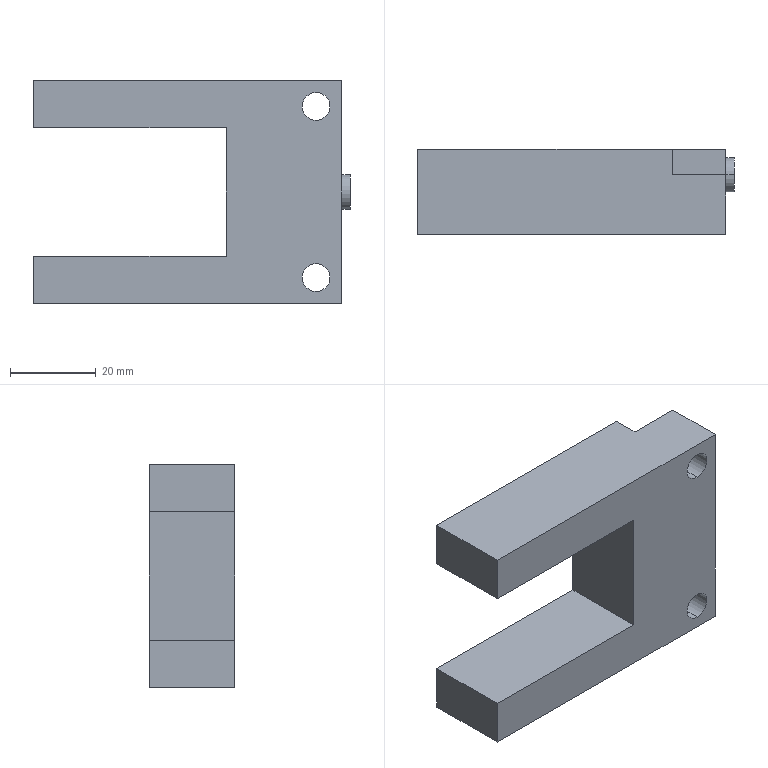Part | 1 solid | 23 faces | box 74 x 20 x 52 mm | volume 45176 mm3 | plane 17 | cylinder 6 | commonest cylinder face diameters 6.5 x4 8 x2
STEP:
#1=CARTESIAN_POINT('',(38.,14.,-4.));
#2=VERTEX_POINT('',#1);
#3=CARTESIAN_POINT('',(38.,14.,4.));
#4=VERTEX_POINT('',#3);
#5=CARTESIAN_POINT('',(38.,14.,0.));
#6=DIRECTION('',(1.,0.,0.));
#7=DIRECTION('',(0.,0.,-1.));
#8=AXIS2_PLACEMENT_3D('',#5,#6,#7);
#9=CIRCLE('',#8,4.);
#10=EDGE_CURVE('',#2,#4,#9,.T.);
#11=ORIENTED_EDGE('',*,*,#10,.F.);
#12=CARTESIAN_POINT('',(36.,14.,-4.));
#13=VERTEX_POINT('',#12);
#14=CARTESIAN_POINT('',(38.,14.,-4.));
#15=DIRECTION('',(-1.,0.,0.));
#16=VECTOR('',#15,1000.);
#17=LINE('',#14,#16);
#18=EDGE_CURVE('',#2,#13,#17,.T.);
#19=ORIENTED_EDGE('',*,*,#18,.T.);
#20=CARTESIAN_POINT('',(36.,14.,4.));
#21=VERTEX_POINT('',#20);
#22=CARTESIAN_POINT('',(36.,14.,0.));
#23=DIRECTION('',(1.,0.,0.));
#24=DIRECTION('',(0.,0.,1.));
#25=AXIS2_PLACEMENT_3D('',#22,#23,#24);
#26=CIRCLE('',#25,4.);
#27=EDGE_CURVE('',#13,#21,#26,.T.);
#28=ORIENTED_EDGE('',*,*,#27,.T.);
#29=CARTESIAN_POINT('',(38.,14.,4.));
#30=DIRECTION('',(-1.,0.,0.));
#31=VECTOR('',#30,1000.);
#32=LINE('',#29,#31);
#33=EDGE_CURVE('',#4,#21,#32,.T.);
#34=ORIENTED_EDGE('',*,*,#33,.F.);
#35=EDGE_LOOP('',(#11,#19,#28,#34));
#36=FACE_OUTER_BOUND('',#35,.T.);
#37=CARTESIAN_POINT('',(38.,14.,0.));
#38=DIRECTION('',(-1.,0.,0.));
#39=DIRECTION('',(0.,0.,1.));
#40=AXIS2_PLACEMENT_3D('',#37,#38,#39);
#41=CYLINDRICAL_SURFACE('',#40,4.);
#42=ADVANCED_FACE('',(#36),#41,.T.);
#43=CARTESIAN_POINT('',(30.,0.,-16.75));
#44=VERTEX_POINT('',#43);
#45=CARTESIAN_POINT('',(30.,0.,-23.25));
#46=VERTEX_POINT('',#45);
#47=CARTESIAN_POINT('',(30.,0.,-20.));
#48=DIRECTION('',(0.,-1.,0.));
#49=DIRECTION('',(0.,0.,-1.));
#50=AXIS2_PLACEMENT_3D('',#47,#48,#49);
#51=CIRCLE('',#50,3.25);
#52=EDGE_CURVE('',#44,#46,#51,.T.);
#53=ORIENTED_EDGE('',*,*,#52,.T.);
#54=CARTESIAN_POINT('',(30.,14.,-23.25));
#55=VERTEX_POINT('',#54);
#56=CARTESIAN_POINT('',(30.,14.,-23.25));
#57=DIRECTION('',(0.,1.,0.));
#58=VECTOR('',#57,1000.);
#59=LINE('',#56,#58);
#60=EDGE_CURVE('',#46,#55,#59,.T.);
#61=ORIENTED_EDGE('',*,*,#60,.T.);
#62=CARTESIAN_POINT('',(30.,14.,-16.75));
#63=VERTEX_POINT('',#62);
#64=CARTESIAN_POINT('',(30.,14.,-20.));
#65=DIRECTION('',(0.,1.,0.));
#66=DIRECTION('',(0.,0.,1.));
#67=AXIS2_PLACEMENT_3D('',#64,#65,#66);
#68=CIRCLE('',#67,3.25);
#69=EDGE_CURVE('',#55,#63,#68,.T.);
#70=ORIENTED_EDGE('',*,*,#69,.T.);
#71=CARTESIAN_POINT('',(30.,14.,-16.75));
#72=DIRECTION('',(0.,1.,0.));
#73=VECTOR('',#72,1000.);
#74=LINE('',#71,#73);
#75=EDGE_CURVE('',#44,#63,#74,.T.);
#76=ORIENTED_EDGE('',*,*,#75,.F.);
#77=EDGE_LOOP('',(#53,#61,#70,#76));
#78=FACE_OUTER_BOUND('',#77,.T.);
#79=CARTESIAN_POINT('',(30.,14.,-20.));
#80=DIRECTION('',(0.,1.,0.));
#81=DIRECTION('',(0.,0.,1.));
#82=AXIS2_PLACEMENT_3D('',#79,#80,#81);
#83=CYLINDRICAL_SURFACE('',#82,3.25);
#84=ADVANCED_FACE('',(#78),#83,.F.);
#85=CARTESIAN_POINT('',(30.,0.,23.25));
#86=VERTEX_POINT('',#85);
#87=CARTESIAN_POINT('',(30.,0.,16.75));
#88=VERTEX_POINT('',#87);
#89=CARTESIAN_POINT('',(30.,0.,20.));
#90=DIRECTION('',(0.,-1.,0.));
#91=DIRECTION('',(0.,0.,-1.));
#92=AXIS2_PLACEMENT_3D('',#89,#90,#91);
#93=CIRCLE('',#92,3.25);
#94=EDGE_CURVE('',#86,#88,#93,.T.);
#95=ORIENTED_EDGE('',*,*,#94,.T.);
#96=CARTESIAN_POINT('',(30.,14.,16.75));
#97=VERTEX_POINT('',#96);
#98=CARTESIAN_POINT('',(30.,14.,16.75));
#99=DIRECTION('',(0.,1.,0.));
#100=VECTOR('',#99,1000.);
#101=LINE('',#98,#100);
#102=EDGE_CURVE('',#88,#97,#101,.T.);
#103=ORIENTED_EDGE('',*,*,#102,.T.);
#104=CARTESIAN_POINT('',(30.,14.,23.25));
#105=VERTEX_POINT('',#104);
#106=CARTESIAN_POINT('',(30.,14.,20.));
#107=DIRECTION('',(0.,1.,0.));
#108=DIRECTION('',(0.,0.,1.));
#109=AXIS2_PLACEMENT_3D('',#106,#107,#108);
#110=CIRCLE('',#109,3.25);
#111=EDGE_CURVE('',#97,#105,#110,.T.);
#112=ORIENTED_EDGE('',*,*,#111,.T.);
#113=CARTESIAN_POINT('',(30.,14.,23.25));
#114=DIRECTION('',(0.,1.,0.));
#115=VECTOR('',#114,1000.);
#116=LINE('',#113,#115);
#117=EDGE_CURVE('',#86,#105,#116,.T.);
#118=ORIENTED_EDGE('',*,*,#117,.F.);
#119=EDGE_LOOP('',(#95,#103,#112,#118));
#120=FACE_OUTER_BOUND('',#119,.T.);
#121=CARTESIAN_POINT('',(30.,14.,20.));
#122=DIRECTION('',(0.,1.,0.));
#123=DIRECTION('',(0.,0.,1.));
#124=AXIS2_PLACEMENT_3D('',#121,#122,#123);
#125=CYLINDRICAL_SURFACE('',#124,3.25);
#126=ADVANCED_FACE('',(#120),#125,.F.);
#127=CARTESIAN_POINT('',(-36.,0.,-26.));
#128=VERTEX_POINT('',#127);
#129=CARTESIAN_POINT('',(-36.,0.,-15.));
#130=VERTEX_POINT('',#129);
#131=CARTESIAN_POINT('',(-36.,0.,26.));
#132=DIRECTION('',(0.,0.,1.));
#133=VECTOR('',#132,1000.);
#134=LINE('',#131,#133);
#135=EDGE_CURVE('',#128,#130,#134,.T.);
#136=ORIENTED_EDGE('',*,*,#135,.T.);
#137=CARTESIAN_POINT('',(-36.,20.,-15.));
#138=VERTEX_POINT('',#137);
#139=CARTESIAN_POINT('',(-36.,0.,-15.));
#140=DIRECTION('',(0.,1.,0.));
#141=VECTOR('',#140,1000.);
#142=LINE('',#139,#141);
#143=EDGE_CURVE('',#130,#138,#142,.T.);
#144=ORIENTED_EDGE('',*,*,#143,.T.);
#145=CARTESIAN_POINT('',(-36.,20.,-26.));
#146=VERTEX_POINT('',#145);
#147=CARTESIAN_POINT('',(-36.,20.,26.));
#148=DIRECTION('',(0.,0.,1.));
#149=VECTOR('',#148,1000.);
#150=LINE('',#147,#149);
#151=EDGE_CURVE('',#146,#138,#150,.T.);
#152=ORIENTED_EDGE('',*,*,#151,.F.);
#153=CARTESIAN_POINT('',(-36.,20.,-26.));
#154=DIRECTION('',(0.,-1.,0.));
#155=VECTOR('',#154,1000.);
#156=LINE('',#153,#155);
#157=EDGE_CURVE('',#146,#128,#156,.T.);
#158=ORIENTED_EDGE('',*,*,#157,.T.);
#159=EDGE_LOOP('',(#136,#144,#152,#158));
#160=FACE_OUTER_BOUND('',#159,.T.);
#161=CARTESIAN_POINT('',(-36.,20.,26.));
#162=DIRECTION('',(1.,0.,0.));
#163=DIRECTION('',(0.,0.,-1.));
#164=AXIS2_PLACEMENT_3D('',#161,#162,#163);
#165=PLANE('',#164);
#166=ADVANCED_FACE('',(#160),#165,.F.);
#167=CARTESIAN_POINT('',(36.,14.,0.));
#168=DIRECTION('',(1.,0.,0.));
#169=DIRECTION('',(0.,0.,1.));
#170=AXIS2_PLACEMENT_3D('',#167,#168,#169);
#171=CIRCLE('',#170,4.);
#172=EDGE_CURVE('',#21,#13,#171,.T.);
#173=ORIENTED_EDGE('',*,*,#172,.F.);
#174=ORIENTED_EDGE('',*,*,#27,.F.);
#175=EDGE_LOOP('',(#173,#174));
#176=FACE_BOUND('',#175,.T.);
#177=CARTESIAN_POINT('',(36.,14.,-13.5));
#178=VERTEX_POINT('',#177);
#179=CARTESIAN_POINT('',(36.,14.,-26.));
#180=VERTEX_POINT('',#179);
#181=CARTESIAN_POINT('',(36.,14.,-26.));
#182=DIRECTION('',(0.,0.,-1.));
#183=VECTOR('',#182,1000.);
#184=LINE('',#181,#183);
#185=EDGE_CURVE('',#178,#180,#184,.T.);
#186=ORIENTED_EDGE('',*,*,#185,.F.);
#187=CARTESIAN_POINT('',(36.,20.,-13.5));
#188=VERTEX_POINT('',#187);
#189=CARTESIAN_POINT('',(36.,14.,-13.5));
#190=DIRECTION('',(0.,1.,0.));
#191=VECTOR('',#190,1000.);
#192=LINE('',#189,#191);
#193=EDGE_CURVE('',#178,#188,#192,.T.);
#194=ORIENTED_EDGE('',*,*,#193,.T.);
#195=CARTESIAN_POINT('',(36.,20.,13.5));
#196=VERTEX_POINT('',#195);
#197=CARTESIAN_POINT('',(36.,20.,26.));
#198=DIRECTION('',(0.,0.,-1.));
#199=VECTOR('',#198,1000.);
#200=LINE('',#197,#199);
#201=EDGE_CURVE('',#196,#188,#200,.T.);
#202=ORIENTED_EDGE('',*,*,#201,.F.);
#203=CARTESIAN_POINT('',(36.,14.,13.5));
#204=VERTEX_POINT('',#203);
#205=CARTESIAN_POINT('',(36.,14.,13.5));
#206=DIRECTION('',(0.,1.,0.));
#207=VECTOR('',#206,1000.);
#208=LINE('',#205,#207);
#209=EDGE_CURVE('',#204,#196,#208,.T.);
#210=ORIENTED_EDGE('',*,*,#209,.F.);
#211=CARTESIAN_POINT('',(36.,14.,26.));
#212=VERTEX_POINT('',#211);
#213=CARTESIAN_POINT('',(36.,14.,26.));
#214=DIRECTION('',(0.,0.,-1.));
#215=VECTOR('',#214,1000.);
#216=LINE('',#213,#215);
#217=EDGE_CURVE('',#212,#204,#216,.T.);
#218=ORIENTED_EDGE('',*,*,#217,.F.);
#219=CARTESIAN_POINT('',(36.,0.,26.));
#220=VERTEX_POINT('',#219);
#221=CARTESIAN_POINT('',(36.,20.,26.));
#222=DIRECTION('',(0.,-1.,0.));
#223=VECTOR('',#222,1000.);
#224=LINE('',#221,#223);
#225=EDGE_CURVE('',#212,#220,#224,.T.);
#226=ORIENTED_EDGE('',*,*,#225,.T.);
#227=CARTESIAN_POINT('',(36.,0.,-26.));
#228=VERTEX_POINT('',#227);
#229=CARTESIAN_POINT('',(36.,0.,26.));
#230=DIRECTION('',(0.,0.,-1.));
#231=VECTOR('',#230,1000.);
#232=LINE('',#229,#231);
#233=EDGE_CURVE('',#220,#228,#232,.T.);
#234=ORIENTED_EDGE('',*,*,#233,.T.);
#235=CARTESIAN_POINT('',(36.,20.,-26.));
#236=DIRECTION('',(0.,-1.,0.));
#237=VECTOR('',#236,1000.);
#238=LINE('',#235,#237);
#239=EDGE_CURVE('',#180,#228,#238,.T.);
#240=ORIENTED_EDGE('',*,*,#239,.F.);
#241=EDGE_LOOP('',(#186,#194,#202,#210,#218,#226,#234,#240));
#242=FACE_OUTER_BOUND('',#241,.T.);
#243=CARTESIAN_POINT('',(36.,20.,26.));
#244=DIRECTION('',(-1.,0.,0.));
#245=DIRECTION('',(0.,0.,1.));
#246=AXIS2_PLACEMENT_3D('',#243,#244,#245);
#247=PLANE('',#246);
#248=ADVANCED_FACE('',(#176,#242),#247,.F.);
#249=CARTESIAN_POINT('',(23.5,20.,-26.));
#250=VERTEX_POINT('',#249);
#251=CARTESIAN_POINT('',(-36.,20.,-26.));
#252=DIRECTION('',(-1.,0.,0.));
#253=VECTOR('',#252,1000.);
#254=LINE('',#251,#253);
#255=EDGE_CURVE('',#250,#146,#254,.T.);
#256=ORIENTED_EDGE('',*,*,#255,.F.);
#257=CARTESIAN_POINT('',(23.5,14.,-26.));
#258=VERTEX_POINT('',#257);
#259=CARTESIAN_POINT('',(23.5,14.,-26.));
#260=DIRECTION('',(0.,1.,0.));
#261=VECTOR('',#260,1000.);
#262=LINE('',#259,#261);
#263=EDGE_CURVE('',#258,#250,#262,.T.);
#264=ORIENTED_EDGE('',*,*,#263,.F.);
#265=CARTESIAN_POINT('',(36.,14.,-26.));
#266=DIRECTION('',(-1.,0.,0.));
#267=VECTOR('',#266,1000.);
#268=LINE('',#265,#267);
#269=EDGE_CURVE('',#180,#258,#268,.T.);
#270=ORIENTED_EDGE('',*,*,#269,.F.);
#271=ORIENTED_EDGE('',*,*,#239,.T.);
#272=CARTESIAN_POINT('',(-36.,0.,-26.));
#273=DIRECTION('',(-1.,0.,0.));
#274=VECTOR('',#273,1000.);
#275=LINE('',#272,#274);
#276=EDGE_CURVE('',#228,#128,#275,.T.);
#277=ORIENTED_EDGE('',*,*,#276,.T.);
#278=ORIENTED_EDGE('',*,*,#157,.F.);
#279=EDGE_LOOP('',(#256,#264,#270,#271,#277,#278));
#280=FACE_OUTER_BOUND('',#279,.T.);
#281=CARTESIAN_POINT('',(-36.,20.,-26.));
#282=DIRECTION('',(0.,0.,1.));
#283=DIRECTION('',(1.,0.,0.));
#284=AXIS2_PLACEMENT_3D('',#281,#282,#283);
#285=PLANE('',#284);
#286=ADVANCED_FACE('',(#280),#285,.F.);
#287=CARTESIAN_POINT('',(-36.,20.,15.));
#288=VERTEX_POINT('',#287);
#289=CARTESIAN_POINT('',(-36.,20.,26.));
#290=VERTEX_POINT('',#289);
#291=CARTESIAN_POINT('',(-36.,20.,26.));
#292=DIRECTION('',(0.,0.,1.));
#293=VECTOR('',#292,1000.);
#294=LINE('',#291,#293);
#295=EDGE_CURVE('',#288,#290,#294,.T.);
#296=ORIENTED_EDGE('',*,*,#295,.F.);
#297=CARTESIAN_POINT('',(-36.,0.,15.));
#298=VERTEX_POINT('',#297);
#299=CARTESIAN_POINT('',(-36.,0.,15.));
#300=DIRECTION('',(0.,1.,0.));
#301=VECTOR('',#300,1000.);
#302=LINE('',#299,#301);
#303=EDGE_CURVE('',#298,#288,#302,.T.);
#304=ORIENTED_EDGE('',*,*,#303,.F.);
#305=CARTESIAN_POINT('',(-36.,0.,26.));
#306=VERTEX_POINT('',#305);
#307=CARTESIAN_POINT('',(-36.,0.,26.));
#308=DIRECTION('',(0.,0.,1.));
#309=VECTOR('',#308,1000.);
#310=LINE('',#307,#309);
#311=EDGE_CURVE('',#298,#306,#310,.T.);
#312=ORIENTED_EDGE('',*,*,#311,.T.);
#313=CARTESIAN_POINT('',(-36.,20.,26.));
#314=DIRECTION('',(0.,-1.,0.));
#315=VECTOR('',#314,1000.);
#316=LINE('',#313,#315);
#317=EDGE_CURVE('',#290,#306,#316,.T.);
#318=ORIENTED_EDGE('',*,*,#317,.F.);
#319=EDGE_LOOP('',(#296,#304,#312,#318));
#320=FACE_OUTER_BOUND('',#319,.T.);
#321=CARTESIAN_POINT('',(-36.,20.,26.));
#322=DIRECTION('',(1.,0.,0.));
#323=DIRECTION('',(0.,0.,-1.));
#324=AXIS2_PLACEMENT_3D('',#321,#322,#323);
#325=PLANE('',#324);
#326=ADVANCED_FACE('',(#320),#325,.F.);
#327=CARTESIAN_POINT('',(23.5,14.,26.));
#328=VERTEX_POINT('',#327);
#329=CARTESIAN_POINT('',(36.,14.,26.));
#330=DIRECTION('',(1.,0.,0.));
#331=VECTOR('',#330,1000.);
#332=LINE('',#329,#331);
#333=EDGE_CURVE('',#328,#212,#332,.T.);
#334=ORIENTED_EDGE('',*,*,#333,.F.);
#335=CARTESIAN_POINT('',(23.5,20.,26.));
#336=VERTEX_POINT('',#335);
#337=CARTESIAN_POINT('',(23.5,14.,26.));
#338=DIRECTION('',(0.,1.,0.));
#339=VECTOR('',#338,1000.);
#340=LINE('',#337,#339);
#341=EDGE_CURVE('',#328,#336,#340,.T.);
#342=ORIENTED_EDGE('',*,*,#341,.T.);
#343=CARTESIAN_POINT('',(-36.,20.,26.));
#344=DIRECTION('',(1.,0.,0.));
#345=VECTOR('',#344,1000.);
#346=LINE('',#343,#345);
#347=EDGE_CURVE('',#290,#336,#346,.T.);
#348=ORIENTED_EDGE('',*,*,#347,.F.);
#349=ORIENTED_EDGE('',*,*,#317,.T.);
#350=CARTESIAN_POINT('',(-36.,0.,26.));
#351=DIRECTION('',(1.,0.,0.));
#352=VECTOR('',#351,1000.);
#353=LINE('',#350,#352);
#354=EDGE_CURVE('',#306,#220,#353,.T.);
#355=ORIENTED_EDGE('',*,*,#354,.T.);
#356=ORIENTED_EDGE('',*,*,#225,.F.);
#357=EDGE_LOOP('',(#334,#342,#348,#349,#355,#356));
#358=FACE_OUTER_BOUND('',#357,.T.);
#359=CARTESIAN_POINT('',(-36.,20.,26.));
#360=DIRECTION('',(0.,0.,-1.));
#361=DIRECTION('',(-1.,0.,0.));
#362=AXIS2_PLACEMENT_3D('',#359,#360,#361);
#363=PLANE('',#362);
#364=ADVANCED_FACE('',(#358),#363,.F.);
#365=ORIENTED_EDGE('',*,*,#201,.T.);
#366=CARTESIAN_POINT('',(23.5,20.,-13.5));
#367=VERTEX_POINT('',#366);
#368=CARTESIAN_POINT('',(36.,20.,-13.5));
#369=DIRECTION('',(1.,0.,0.));
#370=VECTOR('',#369,1000.);
#371=LINE('',#368,#370);
#372=EDGE_CURVE('',#367,#188,#371,.T.);
#373=ORIENTED_EDGE('',*,*,#372,.F.);
#374=CARTESIAN_POINT('',(23.5,20.,-26.));
#375=DIRECTION('',(0.,0.,1.));
#376=VECTOR('',#375,1000.);
#377=LINE('',#374,#376);
#378=EDGE_CURVE('',#250,#367,#377,.T.);
#379=ORIENTED_EDGE('',*,*,#378,.F.);
#380=ORIENTED_EDGE('',*,*,#255,.T.);
#381=ORIENTED_EDGE('',*,*,#151,.T.);
#382=CARTESIAN_POINT('',(9.,20.,-15.));
#383=VERTEX_POINT('',#382);
#384=CARTESIAN_POINT('',(-36.,20.,-15.));
#385=DIRECTION('',(-1.,0.,0.));
#386=VECTOR('',#385,1000.);
#387=LINE('',#384,#386);
#388=EDGE_CURVE('',#383,#138,#387,.T.);
#389=ORIENTED_EDGE('',*,*,#388,.F.);
#390=CARTESIAN_POINT('',(9.,20.,15.));
#391=VERTEX_POINT('',#390);
#392=CARTESIAN_POINT('',(9.,20.,-15.));
#393=DIRECTION('',(0.,0.,-1.));
#394=VECTOR('',#393,1000.);
#395=LINE('',#392,#394);
#396=EDGE_CURVE('',#391,#383,#395,.T.);
#397=ORIENTED_EDGE('',*,*,#396,.F.);
#398=CARTESIAN_POINT('',(-36.,20.,15.));
#399=DIRECTION('',(1.,0.,0.));
#400=VECTOR('',#399,1000.);
#401=LINE('',#398,#400);
#402=EDGE_CURVE('',#288,#391,#401,.T.);
#403=ORIENTED_EDGE('',*,*,#402,.F.);
#404=ORIENTED_EDGE('',*,*,#295,.T.);
#405=ORIENTED_EDGE('',*,*,#347,.T.);
#406=CARTESIAN_POINT('',(23.5,20.,13.5));
#407=VERTEX_POINT('',#406);
#408=CARTESIAN_POINT('',(23.5,20.,26.));
#409=DIRECTION('',(0.,0.,1.));
#410=VECTOR('',#409,1000.);
#411=LINE('',#408,#410);
#412=EDGE_CURVE('',#407,#336,#411,.T.);
#413=ORIENTED_EDGE('',*,*,#412,.F.);
#414=CARTESIAN_POINT('',(36.,20.,13.5));
#415=DIRECTION('',(-1.,0.,0.));
#416=VECTOR('',#415,1000.);
#417=LINE('',#414,#416);
#418=EDGE_CURVE('',#196,#407,#417,.T.);
#419=ORIENTED_EDGE('',*,*,#418,.F.);
#420=EDGE_LOOP('',(#365,#373,#379,#380,#381,#389,#397,#403,#404,#405,#413,#419));
#421=FACE_OUTER_BOUND('',#420,.T.);
#422=CARTESIAN_POINT('',(0.,20.,0.));
#423=DIRECTION('',(0.,-1.,0.));
#424=DIRECTION('',(0.,0.,-1.));
#425=AXIS2_PLACEMENT_3D('',#422,#423,#424);
#426=PLANE('',#425);
#427=ADVANCED_FACE('',(#421),#426,.F.);
#428=ORIENTED_EDGE('',*,*,#52,.F.);
#429=CARTESIAN_POINT('',(30.,0.,-20.));
#430=DIRECTION('',(0.,-1.,0.));
#431=DIRECTION('',(0.,0.,-1.));
#432=AXIS2_PLACEMENT_3D('',#429,#430,#431);
#433=CIRCLE('',#432,3.25);
#434=EDGE_CURVE('',#46,#44,#433,.T.);
#435=ORIENTED_EDGE('',*,*,#434,.F.);
#436=EDGE_LOOP('',(#428,#435));
#437=FACE_BOUND('',#436,.T.);
#438=ORIENTED_EDGE('',*,*,#94,.F.);
#439=CARTESIAN_POINT('',(30.,0.,20.));
#440=DIRECTION('',(0.,-1.,0.));
#441=DIRECTION('',(0.,0.,-1.));
#442=AXIS2_PLACEMENT_3D('',#439,#440,#441);
#443=CIRCLE('',#442,3.25);
#444=EDGE_CURVE('',#88,#86,#443,.T.);
#445=ORIENTED_EDGE('',*,*,#444,.F.);
#446=EDGE_LOOP('',(#438,#445));
#447=FACE_BOUND('',#446,.T.);
#448=CARTESIAN_POINT('',(9.,0.,-15.));
#449=VERTEX_POINT('',#448);
#450=CARTESIAN_POINT('',(-36.,0.,-15.));
#451=DIRECTION('',(-1.,0.,0.));
#452=VECTOR('',#451,1000.);
#453=LINE('',#450,#452);
#454=EDGE_CURVE('',#449,#130,#453,.T.);
#455=ORIENTED_EDGE('',*,*,#454,.T.);
#456=ORIENTED_EDGE('',*,*,#135,.F.);
#457=ORIENTED_EDGE('',*,*,#276,.F.);
#458=ORIENTED_EDGE('',*,*,#233,.F.);
#459=ORIENTED_EDGE('',*,*,#354,.F.);
#460=ORIENTED_EDGE('',*,*,#311,.F.);
#461=CARTESIAN_POINT('',(9.,0.,15.));
#462=VERTEX_POINT('',#461);
#463=CARTESIAN_POINT('',(-36.,0.,15.));
#464=DIRECTION('',(1.,0.,0.));
#465=VECTOR('',#464,1000.);
#466=LINE('',#463,#465);
#467=EDGE_CURVE('',#298,#462,#466,.T.);
#468=ORIENTED_EDGE('',*,*,#467,.T.);
#469=CARTESIAN_POINT('',(9.,0.,-15.));
#470=DIRECTION('',(0.,0.,-1.));
#471=VECTOR('',#470,1000.);
#472=LINE('',#469,#471);
#473=EDGE_CURVE('',#462,#449,#472,.T.);
#474=ORIENTED_EDGE('',*,*,#473,.T.);
#475=EDGE_LOOP('',(#455,#456,#457,#458,#459,#460,#468,#474));
#476=FACE_OUTER_BOUND('',#475,.T.);
#477=CARTESIAN_POINT('',(0.,0.,0.));
#478=DIRECTION('',(0.,-1.,0.));
#479=DIRECTION('',(0.,0.,-1.));
#480=AXIS2_PLACEMENT_3D('',#477,#478,#479);
#481=PLANE('',#480);
#482=ADVANCED_FACE('',(#437,#447,#476),#481,.T.);
#483=ORIENTED_EDGE('',*,*,#388,.T.);
#484=ORIENTED_EDGE('',*,*,#143,.F.);
#485=ORIENTED_EDGE('',*,*,#454,.F.);
#486=CARTESIAN_POINT('',(9.,0.,-15.));
#487=DIRECTION('',(0.,1.,0.));
#488=VECTOR('',#487,1000.);
#489=LINE('',#486,#488);
#490=EDGE_CURVE('',#449,#383,#489,.T.);
#491=ORIENTED_EDGE('',*,*,#490,.T.);
#492=EDGE_LOOP('',(#483,#484,#485,#491));
#493=FACE_OUTER_BOUND('',#492,.T.);
#494=CARTESIAN_POINT('',(-36.,0.,-15.));
#495=DIRECTION('',(0.,0.,-1.));
#496=DIRECTION('',(-1.,0.,0.));
#497=AXIS2_PLACEMENT_3D('',#494,#495,#496);
#498=PLANE('',#497);
#499=ADVANCED_FACE('',(#493),#498,.F.);
#500=ORIENTED_EDGE('',*,*,#396,.T.);
#501=ORIENTED_EDGE('',*,*,#490,.F.);
#502=ORIENTED_EDGE('',*,*,#473,.F.);
#503=CARTESIAN_POINT('',(9.,0.,15.));
#504=DIRECTION('',(0.,1.,0.));
#505=VECTOR('',#504,1000.);
#506=LINE('',#503,#505);
#507=EDGE_CURVE('',#462,#391,#506,.T.);
#508=ORIENTED_EDGE('',*,*,#507,.T.);
#509=EDGE_LOOP('',(#500,#501,#502,#508));
#510=FACE_OUTER_BOUND('',#509,.T.);
#511=CARTESIAN_POINT('',(9.,0.,-15.));
#512=DIRECTION('',(1.,0.,0.));
#513=DIRECTION('',(0.,0.,-1.));
#514=AXIS2_PLACEMENT_3D('',#511,#512,#513);
#515=PLANE('',#514);
#516=ADVANCED_FACE('',(#510),#515,.F.);
#517=ORIENTED_EDGE('',*,*,#402,.T.);
#518=ORIENTED_EDGE('',*,*,#507,.F.);
#519=ORIENTED_EDGE('',*,*,#467,.F.);
#520=ORIENTED_EDGE('',*,*,#303,.T.);
#521=EDGE_LOOP('',(#517,#518,#519,#520));
#522=FACE_OUTER_BOUND('',#521,.T.);
#523=CARTESIAN_POINT('',(-36.,0.,15.));
#524=DIRECTION('',(0.,0.,1.));
#525=DIRECTION('',(1.,0.,0.));
#526=AXIS2_PLACEMENT_3D('',#523,#524,#525);
#527=PLANE('',#526);
#528=ADVANCED_FACE('',(#522),#527,.F.);
#529=ORIENTED_EDGE('',*,*,#412,.T.);
#530=ORIENTED_EDGE('',*,*,#341,.F.);
#531=CARTESIAN_POINT('',(23.5,14.,13.5));
#532=VERTEX_POINT('',#531);
#533=CARTESIAN_POINT('',(23.5,14.,26.));
#534=DIRECTION('',(0.,0.,1.));
#535=VECTOR('',#534,1000.);
#536=LINE('',#533,#535);
#537=EDGE_CURVE('',#532,#328,#536,.T.);
#538=ORIENTED_EDGE('',*,*,#537,.F.);
#539=CARTESIAN_POINT('',(23.5,14.,13.5));
#540=DIRECTION('',(0.,1.,0.));
#541=VECTOR('',#540,1000.);
#542=LINE('',#539,#541);
#543=EDGE_CURVE('',#532,#407,#542,.T.);
#544=ORIENTED_EDGE('',*,*,#543,.T.);
#545=EDGE_LOOP('',(#529,#530,#538,#544));
#546=FACE_OUTER_BOUND('',#545,.T.);
#547=CARTESIAN_POINT('',(23.5,14.,26.));
#548=DIRECTION('',(-1.,0.,0.));
#549=DIRECTION('',(0.,0.,1.));
#550=AXIS2_PLACEMENT_3D('',#547,#548,#549);
#551=PLANE('',#550);
#552=ADVANCED_FACE('',(#546),#551,.F.);
#553=ORIENTED_EDGE('',*,*,#418,.T.);
#554=ORIENTED_EDGE('',*,*,#543,.F.);
#555=CARTESIAN_POINT('',(36.,14.,13.5));
#556=DIRECTION('',(-1.,0.,0.));
#557=VECTOR('',#556,1000.);
#558=LINE('',#555,#557);
#559=EDGE_CURVE('',#204,#532,#558,.T.);
#560=ORIENTED_EDGE('',*,*,#559,.F.);
#561=ORIENTED_EDGE('',*,*,#209,.T.);
#562=EDGE_LOOP('',(#553,#554,#560,#561));
#563=FACE_OUTER_BOUND('',#562,.T.);
#564=CARTESIAN_POINT('',(36.,14.,13.5));
#565=DIRECTION('',(0.,0.,-1.));
#566=DIRECTION('',(-1.,0.,0.));
#567=AXIS2_PLACEMENT_3D('',#564,#565,#566);
#568=PLANE('',#567);
#569=ADVANCED_FACE('',(#563),#568,.F.);
#570=CARTESIAN_POINT('',(30.,14.,20.));
#571=DIRECTION('',(0.,1.,0.));
#572=DIRECTION('',(0.,0.,1.));
#573=AXIS2_PLACEMENT_3D('',#570,#571,#572);
#574=CIRCLE('',#573,3.25);
#575=EDGE_CURVE('',#105,#97,#574,.T.);
#576=ORIENTED_EDGE('',*,*,#575,.F.);
#577=ORIENTED_EDGE('',*,*,#111,.F.);
#578=EDGE_LOOP('',(#576,#577));
#579=FACE_BOUND('',#578,.T.);
#580=ORIENTED_EDGE('',*,*,#333,.T.);
#581=ORIENTED_EDGE('',*,*,#217,.T.);
#582=ORIENTED_EDGE('',*,*,#559,.T.);
#583=ORIENTED_EDGE('',*,*,#537,.T.);
#584=EDGE_LOOP('',(#580,#581,#582,#583));
#585=FACE_OUTER_BOUND('',#584,.T.);
#586=CARTESIAN_POINT('',(0.,14.,0.));
#587=DIRECTION('',(0.,-1.,0.));
#588=DIRECTION('',(0.,0.,-1.));
#589=AXIS2_PLACEMENT_3D('',#586,#587,#588);
#590=PLANE('',#589);
#591=ADVANCED_FACE('',(#579,#585),#590,.F.);
#592=ORIENTED_EDGE('',*,*,#372,.T.);
#593=ORIENTED_EDGE('',*,*,#193,.F.);
#594=CARTESIAN_POINT('',(23.5,14.,-13.5));
#595=VERTEX_POINT('',#594);
#596=CARTESIAN_POINT('',(36.,14.,-13.5));
#597=DIRECTION('',(1.,0.,0.));
#598=VECTOR('',#597,1000.);
#599=LINE('',#596,#598);
#600=EDGE_CURVE('',#595,#178,#599,.T.);
#601=ORIENTED_EDGE('',*,*,#600,.F.);
#602=CARTESIAN_POINT('',(23.5,14.,-13.5));
#603=DIRECTION('',(0.,1.,0.));
#604=VECTOR('',#603,1000.);
#605=LINE('',#602,#604);
#606=EDGE_CURVE('',#595,#367,#605,.T.);
#607=ORIENTED_EDGE('',*,*,#606,.T.);
#608=EDGE_LOOP('',(#592,#593,#601,#607));
#609=FACE_OUTER_BOUND('',#608,.T.);
#610=CARTESIAN_POINT('',(36.,14.,-13.5));
#611=DIRECTION('',(0.,0.,1.));
#612=DIRECTION('',(1.,0.,0.));
#613=AXIS2_PLACEMENT_3D('',#610,#611,#612);
#614=PLANE('',#613);
#615=ADVANCED_FACE('',(#609),#614,.F.);
#616=ORIENTED_EDGE('',*,*,#378,.T.);
#617=ORIENTED_EDGE('',*,*,#606,.F.);
#618=CARTESIAN_POINT('',(23.5,14.,-26.));
#619=DIRECTION('',(0.,0.,1.));
#620=VECTOR('',#619,1000.);
#621=LINE('',#618,#620);
#622=EDGE_CURVE('',#258,#595,#621,.T.);
#623=ORIENTED_EDGE('',*,*,#622,.F.);
#624=ORIENTED_EDGE('',*,*,#263,.T.);
#625=EDGE_LOOP('',(#616,#617,#623,#624));
#626=FACE_OUTER_BOUND('',#625,.T.);
#627=CARTESIAN_POINT('',(23.5,14.,-26.));
#628=DIRECTION('',(-1.,0.,0.));
#629=DIRECTION('',(0.,0.,1.));
#630=AXIS2_PLACEMENT_3D('',#627,#628,#629);
#631=PLANE('',#630);
#632=ADVANCED_FACE('',(#626),#631,.F.);
#633=CARTESIAN_POINT('',(30.,14.,-20.));
#634=DIRECTION('',(0.,1.,0.));
#635=DIRECTION('',(0.,0.,1.));
#636=AXIS2_PLACEMENT_3D('',#633,#634,#635);
#637=CIRCLE('',#636,3.25);
#638=EDGE_CURVE('',#63,#55,#637,.T.);
#639=ORIENTED_EDGE('',*,*,#638,.F.);
#640=ORIENTED_EDGE('',*,*,#69,.F.);
#641=EDGE_LOOP('',(#639,#640));
#642=FACE_BOUND('',#641,.T.);
#643=ORIENTED_EDGE('',*,*,#185,.T.);
#644=ORIENTED_EDGE('',*,*,#269,.T.);
#645=ORIENTED_EDGE('',*,*,#622,.T.);
#646=ORIENTED_EDGE('',*,*,#600,.T.);
#647=EDGE_LOOP('',(#643,#644,#645,#646));
#648=FACE_OUTER_BOUND('',#647,.T.);
#649=CARTESIAN_POINT('',(0.,14.,0.));
#650=DIRECTION('',(0.,-1.,0.));
#651=DIRECTION('',(0.,0.,-1.));
#652=AXIS2_PLACEMENT_3D('',#649,#650,#651);
#653=PLANE('',#652);
#654=ADVANCED_FACE('',(#642,#648),#653,.F.);
#655=ORIENTED_EDGE('',*,*,#102,.F.);
#656=ORIENTED_EDGE('',*,*,#444,.T.);
#657=ORIENTED_EDGE('',*,*,#117,.T.);
#658=ORIENTED_EDGE('',*,*,#575,.T.);
#659=EDGE_LOOP('',(#655,#656,#657,#658));
#660=FACE_OUTER_BOUND('',#659,.T.);
#661=CARTESIAN_POINT('',(30.,14.,20.));
#662=DIRECTION('',(0.,1.,0.));
#663=DIRECTION('',(0.,0.,1.));
#664=AXIS2_PLACEMENT_3D('',#661,#662,#663);
#665=CYLINDRICAL_SURFACE('',#664,3.25);
#666=ADVANCED_FACE('',(#660),#665,.F.);
#667=ORIENTED_EDGE('',*,*,#60,.F.);
#668=ORIENTED_EDGE('',*,*,#434,.T.);
#669=ORIENTED_EDGE('',*,*,#75,.T.);
#670=ORIENTED_EDGE('',*,*,#638,.T.);
#671=EDGE_LOOP('',(#667,#668,#669,#670));
#672=FACE_OUTER_BOUND('',#671,.T.);
#673=CARTESIAN_POINT('',(30.,14.,-20.));
#674=DIRECTION('',(0.,1.,0.));
#675=DIRECTION('',(0.,0.,1.));
#676=AXIS2_PLACEMENT_3D('',#673,#674,#675);
#677=CYLINDRICAL_SURFACE('',#676,3.25);
#678=ADVANCED_FACE('',(#672),#677,.F.);
#679=ORIENTED_EDGE('',*,*,#18,.F.);
#680=CARTESIAN_POINT('',(38.,14.,0.));
#681=DIRECTION('',(1.,0.,0.));
#682=DIRECTION('',(0.,0.,-1.));
#683=AXIS2_PLACEMENT_3D('',#680,#681,#682);
#684=CIRCLE('',#683,4.);
#685=EDGE_CURVE('',#4,#2,#684,.T.);
#686=ORIENTED_EDGE('',*,*,#685,.F.);
#687=ORIENTED_EDGE('',*,*,#33,.T.);
#688=ORIENTED_EDGE('',*,*,#172,.T.);
#689=EDGE_LOOP('',(#679,#686,#687,#688));
#690=FACE_OUTER_BOUND('',#689,.T.);
#691=CARTESIAN_POINT('',(38.,14.,0.));
#692=DIRECTION('',(-1.,0.,0.));
#693=DIRECTION('',(0.,0.,1.));
#694=AXIS2_PLACEMENT_3D('',#691,#692,#693);
#695=CYLINDRICAL_SURFACE('',#694,4.);
#696=ADVANCED_FACE('',(#690),#695,.T.);
#697=ORIENTED_EDGE('',*,*,#685,.T.);
#698=ORIENTED_EDGE('',*,*,#10,.T.);
#699=EDGE_LOOP('',(#697,#698));
#700=FACE_OUTER_BOUND('',#699,.T.);
#701=CARTESIAN_POINT('',(38.,14.,0.));
#702=DIRECTION('',(1.,0.,0.));
#703=DIRECTION('',(0.,0.,-1.));
#704=AXIS2_PLACEMENT_3D('',#701,#702,#703);
#705=PLANE('',#704);
#706=ADVANCED_FACE('',(#700),#705,.T.);
#707=CLOSED_SHELL('',(#42,#84,#126,#166,#248,#286,#326,#364,#427,#482,#499,#516,#528,#552,#569,#591,#615,#632,#654,#666,#678,#696,#706));
#708=MANIFOLD_SOLID_BREP('',#707);
#709=CARTESIAN_POINT('',(0.,0.,0.));
#710=DIRECTION('',(0.,0.,1.));
#711=DIRECTION('',(1.,0.,0.));
#712=AXIS2_PLACEMENT_3D('',#709,#710,#711);
#713=(LENGTH_UNIT()NAMED_UNIT(*)SI_UNIT(.MILLI.,.METRE.));
#714=UNCERTAINTY_MEASURE_WITH_UNIT(LENGTH_MEASURE(0.00001),#713,'','');
#715=(NAMED_UNIT(*)PLANE_ANGLE_UNIT()SI_UNIT($,.RADIAN.));
#716=(NAMED_UNIT(*)SI_UNIT($,.STERADIAN.)SOLID_ANGLE_UNIT());
#717=(GEOMETRIC_REPRESENTATION_CONTEXT(3)GLOBAL_UNCERTAINTY_ASSIGNED_CONTEXT((#714))GLOBAL_UNIT_ASSIGNED_CONTEXT((#713,#715,#716))REPRESENTATION_CONTEXT('',''));
#718=ADVANCED_BREP_SHAPE_REPRESENTATION('',(#708,#712),#717);